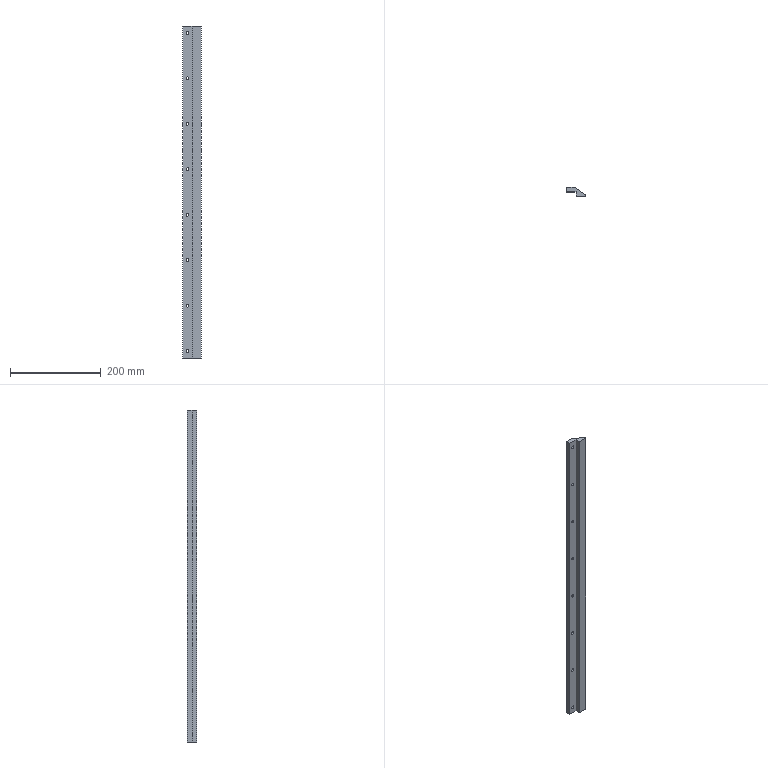NC program | NX | posted with a generic post | part box 40 x 20 x 730 mm
Whole program:
N10 G17 G21 G94 G90
(FLOOR_WALL_1 , TOOL : D10)
N12 T15 M6
N14 G54
N16 G17 G0 G90 X4.33 Y-26.5 B0. C0. S9500 M3
N18 G43 Z30. H15
N20 Z0.01
N22 G94 G1 Z-0.99 F3000.
N24 X0.866 Y-20.5
N26 G3 X0. Y-20. R1.
N28 G1 X-365.
N30 Y-5.1
N32 X365.
N34 Y-20.
N36 X0.
N38 Y-13.
N40 X-358.
N42 Y-12.1
N44 X358.
N46 Y-13.
N48 X0.
N50 G3 X-0.866 Y-13.5 R1.
N52 G1 Z0.01
N54 G0 X4.33 Y-26.5 Z-0.98
N56 G1 Z-1.98
N58 X0.866 Y-20.5
N60 G3 X0. Y-20. R1.
N62 G1 X-365.
N64 Y-5.1
N66 X365.
N68 Y-20.
N70 X0.
N72 Y-13.
N74 X-358.
N76 Y-12.1
N78 X358.
N80 Y-13.
N82 X0.
N84 G3 X-0.866 Y-13.5 R1.
N86 G1 Z-0.98
N88 G0 X4.33 Y-26.5 Z-1.97
N90 G1 Z-2.97
N92 X0.866 Y-20.5
N94 G3 X0. Y-20. R1.
N96 G1 X-365.
N98 Y-5.1
N100 X365.
N102 Y-20.
N104 X0.
N106 Y-13.
N108 X-358.
N110 Y-12.1
N112 X358.
N114 Y-13.
N116 X0.
N118 G3 X-0.866 Y-13.5 R1.
N120 G1 Z-1.97
N122 G0 X4.33 Y-26.5 Z-2.96
N124 G1 Z-3.96
N126 X0.866 Y-20.5
N128 G3 X0. Y-20. R1.
N130 G1 X-365.
N132 Y-5.1
N134 X365.
N136 Y-20.
N138 X0.
N140 Y-13.
N142 X-358.
N144 Y-12.1
N146 X358.
N148 Y-13.
N150 X0.
N152 G3 X-0.866 Y-13.5 R1.
N154 G1 Z-2.96
N156 G0 X4.33 Y-26.5 Z-3.95
N158 G1 Z-4.95
N160 X0.866 Y-20.5
N162 G3 X0. Y-20. R1.
N164 G1 X-365.
N166 Y-5.1
N168 X365.
N170 Y-20.
N172 X0.
N174 Y-13.
N176 X-358.
N178 Y-12.1
N180 X358.
N182 Y-13.
N184 X0.
N186 G3 X-0.866 Y-13.5 R1.
N188 G1 Z-3.95
N190 G0 X4.33 Y-26.5 Z-4.94
N192 G1 Z-5.94
N194 X0.866 Y-20.5
N196 G3 X0. Y-20. R1.
N198 G1 X-365.
N200 Y-5.1
N202 X365.
N204 Y-20.
N206 X0.
N208 Y-13.
N210 X-358.
N212 Y-12.1
N214 X358.
N216 Y-13.
N218 X0.
N220 G3 X-0.866 Y-13.5 R1.
N222 G1 Z-4.94
N224 G0 X4.33 Y-26.5 Z-5.93
N226 G1 Z-6.93
N228 X0.866 Y-20.5
N230 G3 X0. Y-20. R1.
N232 G1 X-365.
N234 Y-5.1
N236 X365.
N238 Y-20.
N240 X0.
N242 Y-13.
N244 X-358.
N246 Y-12.1
N248 X358.
N250 Y-13.
N252 X0.
N254 G3 X-0.866 Y-13.5 R1.
N256 G1 Z-5.93
N258 G0 X4.33 Y-26.5 Z-6.92
N260 G1 Z-7.92
N262 X0.866 Y-20.5
N264 G3 X0. Y-20. R1.
N266 G1 X-365.
N268 Y-5.1
N270 X365.
N272 Y-20.
N274 X0.
N276 Y-13.
N278 X-358.
N280 Y-12.1
N282 X358.
N284 Y-13.
N286 X0.
N288 G3 X-0.866 Y-13.5 R1.
N290 G1 Z-6.92
N292 G0 X4.33 Y-26.5 Z-7.91
N294 G1 Z-8.91
N296 X0.866 Y-20.5
N298 G3 X0. Y-20. R1.
N300 G1 X-365.
N302 Y-5.1
N304 X365.
N306 Y-20.
N308 X0.
N310 Y-13.
N312 X-358.
N314 Y-12.1
N316 X358.
N318 Y-13.
N320 X0.
N322 G3 X-0.866 Y-13.5 R1.
N324 G1 Z-7.91
N326 G0 X4.33 Y-26.5 Z-8.9
N328 G1 Z-9.9
N330 X0.866 Y-20.5
N332 G3 X0. Y-20. R1.
N334 G1 X-365.
N336 Y-5.1
N338 X365.
N340 Y-20.
N342 X0.
N344 Y-13.
N346 X-358.
N348 Y-12.1
N350 X358.
N352 Y-13.
N354 X0.
N356 G3 X-0.866 Y-13.5 R1.
N358 G1 Z-8.9
N360 G0 Z30.
N362 M5
(FLOOR_WALL_1_COPY , TOOL : D10JING)
N364 T14 M6
N366 G54
N368 G17 G0 G90 X371.5 Y-21.595 B0. C0. S9500 M3
N370 G43 Z30. H14
N372 Z-9.
N374 G94 G1 Z-10. F1500.
N376 X370.866 Y-20.497
N378 G3 X370. Y-19.997 R1.
N380 G1 X-370.
N382 Y-15.165
N384 X370.
N386 Y-10.332
N388 X-370.
N390 Y-5.5
N392 X370.
N394 G2 X370.866 Y-6. R1.
N396 G1 X371.5 Y-7.098
N398 Z-9.
N400 G0 Y-6.598
N402 G1 Z-10.
N404 X370.866 Y-5.5
N406 G3 X370. Y-5. R1.
N408 G1 X-370.
N410 G3 X-370.866 Y-5.5 R1.
N412 G1 X-371.5 Y-6.598
N414 Z-9.
N416 G0 Z30.
N418 M5
(DRILLING , TOOL : D6A45)
N420 T01 M6
N422 G54
N424 G17 G0 G90 X-350. Y-10. B0. C0. S9500 M3
N426 G43 Z30. H1
N428 G94 G81 G98 Z-11. F250. R-7.
N430 X-250.
N432 X-150.
N434 X-50.
N436 X50.
N438 X150.
N440 X250.
N442 X350.
N444 G80
N446 G0 X350. Y-10. Z30.
N448 M5
(DRILLING_COPY_COPY , TOOL : 6.2ZT)
N450 T16 M6
N452 G54
N454 G17 G0 G90 X-350. Y-10. B0. C0. S2000 M3
N456 G43 Z30. H16
N458 G94 G83 G98 Z-23.363 F150. Q2. R-7.
N460 X-250.
N462 X-150.
N464 X-50.
N466 X50.
N468 X150.
N470 X250.
N472 X350.
N474 G80
N476 G0 X350. Y-10. Z30.
N478 M5
(PLANAR_MILL , TOOL : D6A45)
N480 T01 M6
N482 G54
N484 G17 G0 G90 X365.866 Y-1.4 B0. C0. S9500 M3
N486 G43 Z30. H1
N488 Z0.5
N490 G94 G1 Z-1. F1250.
N492 G3 X365. Y-0.9 R1.
N494 G1 X-365.
N496 G3 X-365.866 Y-1.4 R1.
N498 G1 Z0.5
N500 G0 Z30.
(PLANAR_MILL_COPY , TOOL : D6A45)
N502 X-350.454 Y-10.891
N504 Z-9.5
N506 G1 Z-11.
N508 X-350.866 Y-11.7
N510 G3 X-350. Y-12.2 R1.
N512 X-347.8 Y-10. R2.2
N514 X-350. Y-12.2 R-2.2
N516 X-349.134 Y-11.7 R1.
N518 G1 X-349.546 Y-10.891
N520 Z-9.5
N522 G0 Z30.
N524 X-250.454
N526 Z-9.5
N528 G1 Z-11.
N530 X-250.866 Y-11.7
N532 G3 X-250. Y-12.2 R1.
N534 X-247.8 Y-10. R2.2
N536 X-250. Y-12.2 R-2.2
N538 X-249.134 Y-11.7 R1.
N540 G1 X-249.546 Y-10.891
N542 Z-9.5
N544 G0 Z30.
N546 X-150.454
N548 Z-9.5
N550 G1 Z-11.
N552 X-150.866 Y-11.7
N554 G3 X-150. Y-12.2 R1.
N556 X-147.8 Y-10. R2.2
N558 X-150. Y-12.2 R-2.2
N560 X-149.134 Y-11.7 R1.
N562 G1 X-149.546 Y-10.891
N564 Z-9.5
N566 G0 Z30.
N568 X-50.454
N570 Z-9.5
N572 G1 Z-11.
N574 X-50.866 Y-11.7
N576 G3 X-50. Y-12.2 R1.
N578 X-47.8 Y-10. R2.2
N580 X-50. Y-12.2 R-2.2
N582 X-49.134 Y-11.7 R1.
N584 G1 X-49.546 Y-10.891
N586 Z-9.5
N588 G0 Z30.
N590 X367.313 Y-4.092
N592 Z-9.5
N594 G1 Z-11.
N596 X366.865 Y-3.643
N598 G3 X365.9 Y-3.382 R1.
N600 G1 Y-19.9
N602 G2 X364.9 Y-20.9 R1.
N604 G1 X-364.9
N606 G2 X-365.9 Y-19.9 R1.
N608 G1 Y-3.382
N610 G3 X-366.865 Y-3.643 R1.
N612 G1 X-367.313 Y-4.092
N614 Z-9.5
N616 G0 Z30.
N618 X49.546 Y-10.891
N620 Z-9.5
N622 G1 Z-11.
N624 X49.134 Y-11.7
N626 G3 X50. Y-12.2 R1.
N628 X52.2 Y-10. R2.2
N630 X50. Y-12.2 R-2.2
N632 X50.866 Y-11.7 R1.
N634 G1 X50.454 Y-10.891
N636 Z-9.5
N638 G0 Z30.
N640 X149.546
N642 Z-9.5
N644 G1 Z-11.
N646 X149.134 Y-11.7
N648 G3 X150. Y-12.2 R1.
N650 X152.2 Y-10. R2.2
N652 X150. Y-12.2 R-2.2
N654 X150.866 Y-11.7 R1.
N656 G1 X150.454 Y-10.891
N658 Z-9.5
N660 G0 Z30.
N662 X249.546
N664 Z-9.5
N666 G1 Z-11.
N668 X249.134 Y-11.7
N670 G3 X250. Y-12.2 R1.
N672 X252.2 Y-10. R2.2
N674 X250. Y-12.2 R-2.2
N676 X250.866 Y-11.7 R1.
N678 G1 X250.454 Y-10.891
N680 Z-9.5
N682 G0 Z30.
N684 X349.546
N686 Z-9.5
N688 G1 Z-11.
N690 X349.134 Y-11.7
N692 G3 X350. Y-12.2 R1.
N694 X352.2 Y-10. R2.2
N696 X350. Y-12.2 R-2.2
N698 X350.866 Y-11.7 R1.
N700 G1 X350.454 Y-10.891
N702 Z-9.5
N704 G0 Z30.
N706 M5
N708 M2